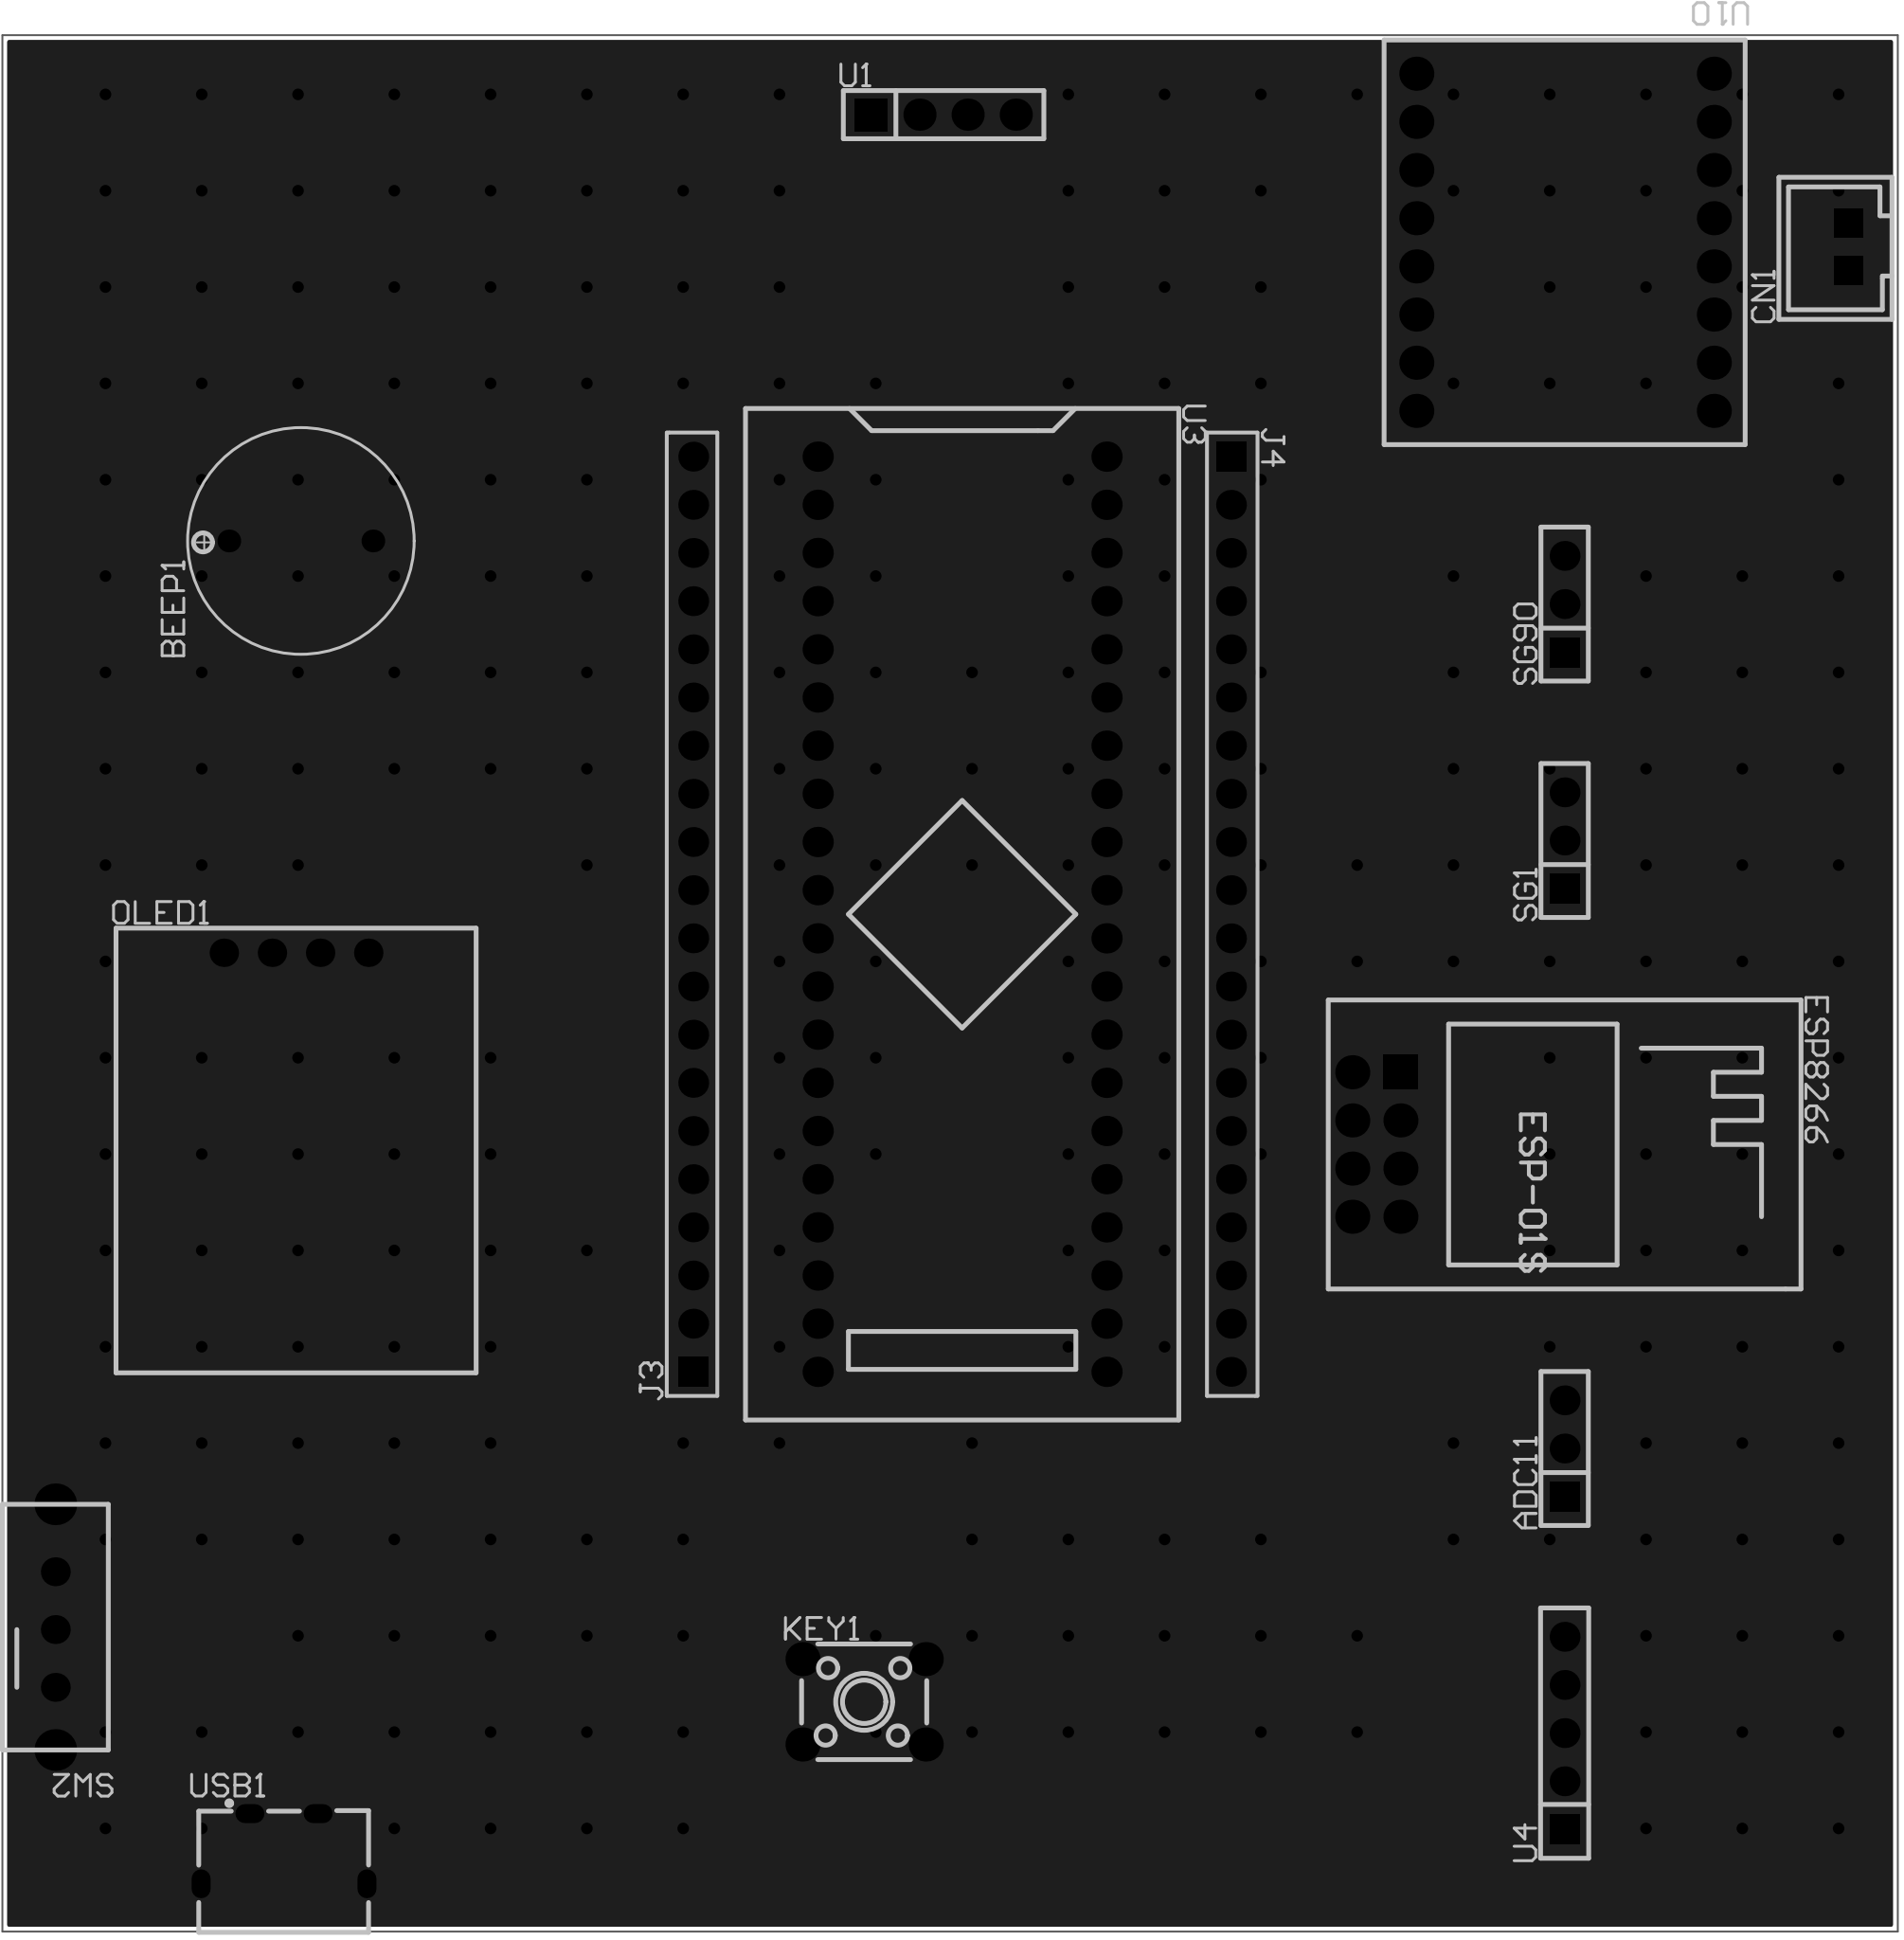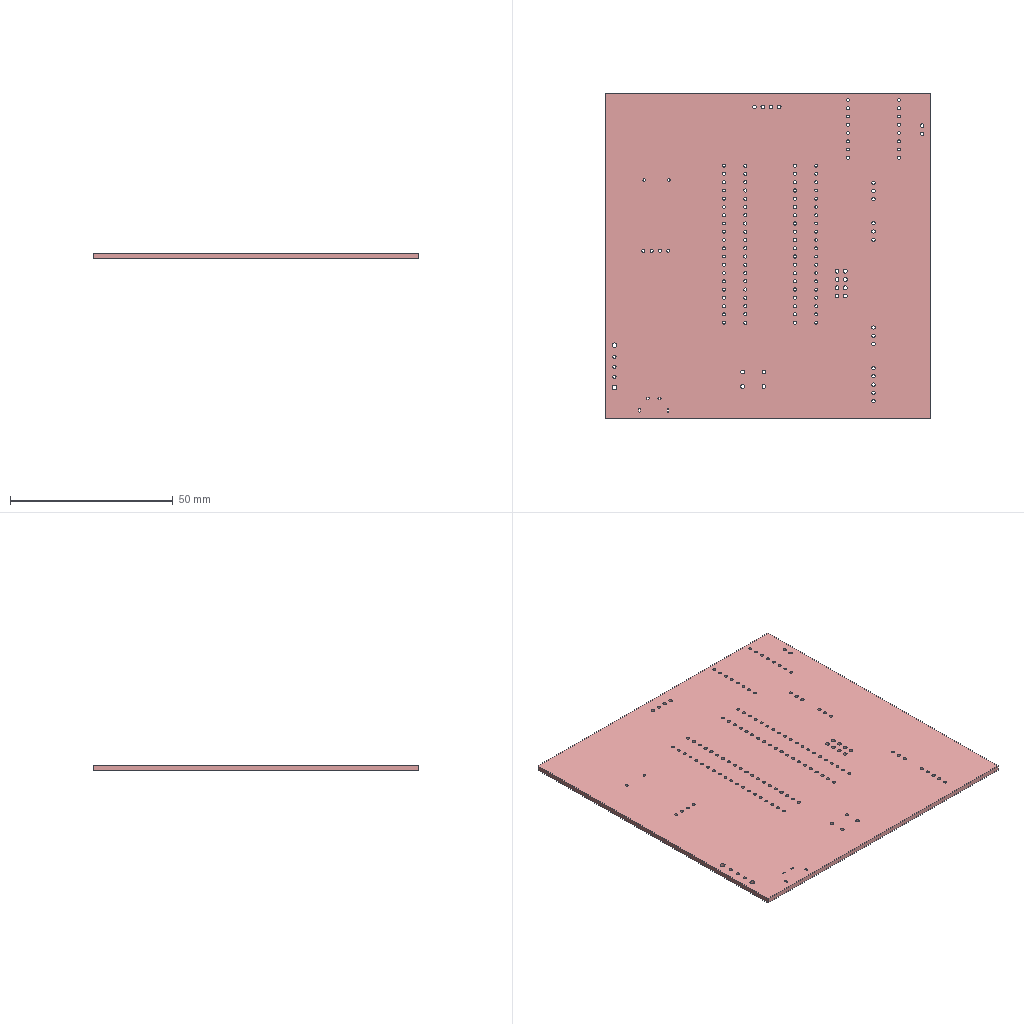Circuit board layout | Altium Designer | box 100 x 100 x 1.6 mm
Layer stack:
# Altium Designer layer stack of  (unit mm; dielectric type: 0 none, 1 core, 2 prepreg, 3 surface material)
index,name,kind,layer,copper_thickness_mm,dielectric_type,dielectric_thickness_mm,dielectric_material,dielectric_constant
0,Top Paste Mask Layer,other,,,,,,
1,Top Silkscreen Layer,other,,,,,,
2,Top Solder Mask Layer,dielectric,,,3,0.01,,3.3
3,Top Layer,copper,Top Layer,0.035,,,,
4,Dielectric1,dielectric,,,3,1.51,FR4,4.5
5,Bottom Layer,copper,Bottom Layer,0.035,,,,
6,Bottom Solder Mask Layer,dielectric,,,3,0.01,,3.3
7,Bottom Silkscreen Layer,other,,,,,,
8,Bottom Paste Mask Layer,other,,,,,,
# drill layer pairs: low layer,high layer
drill_pair,Top Layer,Bottom Layer
Part placement:
Designator,Comment,Layer,Footprint,Center-X(mm),Center-Y(mm),Rotation
ADC11,MQ135,TopLayer,HDR-TH_3P-P2.54-V-F,164.719,108.48,90
BEEP1,Buzzer,TopLayer,BUZ-TH_BD11.8-P7.60_XHXDZ-TMB12065,98.044,156.337,90
CN1,XH2.54-2PIN-straight pin,TopLayer,CONN-TH_XH2.54-2P,179.705,171.831,90
ESP8266,ESP-01S module,TopLayer,WIFIM-TH_ESP-01S,154.788,124.51,270
J3,HDR-M-2.54_1x20,TopLayer,HDR-M-2.54_1X20,118.745,136.652,90
J4,HDR-M-2.54_1x20,TopLayer,HDR-M-2.54_1X20,147.119,136.652,270
KEY1,K4-6×6_TH,TopLayer,KEY-TH_4P-L6.0-W6.0-P4.50-LS6.5,127.762,95.123,0
OLED1,0.96 OLED IIC COPY,TopLayer,OLED-TH_4P-L23.44-W19.0_ER-OLEDM0.66-1W-I2C,97.79,134.62,0
SG1,Servo,TopLayer,HDR-TH_3P-P2.54-V-F,164.719,140.541,90
SG90,Servo,TopLayer,HDR-TH_3P-P2.54-V-F,164.719,153.009,90
SW2,SK-12E12-G5,TopLayer,SW-TH_SK-12E12-G5,85.09,99.06,180
U1,HX711,TopLayer,HDR-TH_4P-P2.54-V-F,131.953,178.816,0
U3,STM32F103C8T6-Card,TopLayer,CONN-TH_L53.3-W22.9_STM32F103C8T6-CARD,132.932,136.652,270
U4,Clock DS1302,TopLayer,HDR-TH_5P-P2.54-V-F,164.719,93.472,90
U10,TB6612FNG,TopLayer,tb6612,164.744,172.085,180
USB1,KH-TYPE-C-2P,TopLayer,USB-SMD_KH-TYPE-C-2P,97.155,87.376,0
Pad and via stacks:
# Altium Designer via and pad stacks of  (unit mm). Each distinct definition once, with the count of objects using it.
# via: kind,start_layer,end_layer,hole_mm,diameter_mm,mode(0 simple;1 top-mid-bottom;2 full stack),diameter_per_layer,count,example_net
# pad: kind,layer,hole_mm,hole_type(0 round;1 square;2 slot),plating,top_size,top_shape(1 round;2 rect;3 octagon;9 rounded rect),mid_size,bottom_size,mode,footprint,size_per_layer,count,example
pad,Multi-Layer,1.02,0,plated,1.575x1.575,1,1.575x1.575,1.575x1.575,0,HDR-TH_3P-P2.54-V-F,,6,ADC11.3
pad,Multi-Layer,1.02,0,plated,1.575x1.575,2,1.575x1.575,1.575x1.575,0,HDR-TH_3P-P2.54-V-F,,3,ADC11.1
pad,Multi-Layer,0.801,0,plated,1.202x1.202,1,1.202x1.202,1.202x1.202,0,BUZ-TH_BD11.8-P7.60_XHXDZ-TMB12065,,2,BEEP1.1
pad,Multi-Layer,1,2,plated,1.524x1.524,2,1.524x1.524,1.524x1.524,0,CONN-TH_XH2.54-2P,,2,CN1.1
pad,Multi-Layer,1.2,0,plated,1.8x1.8,2,1.8x1.8,1.8x1.8,0,WIFIM-TH_ESP-01S,,1,ESP8266.1
pad,Multi-Layer,1.2,0,plated,1.8x1.8,1,1.8x1.8,1.8x1.8,0,WIFIM-TH_ESP-01S,,7,ESP8266.2
pad,Multi-Layer,0.889,0,plated,1.575x1.575,1,1.575x1.575,1.575x1.575,0,HDR-M-2.54_1X20,,38,J3.20
pad,Multi-Layer,0.889,0,plated,1.575x1.575,2,1.575x1.575,1.575x1.575,0,HDR-M-2.54_1X20,,2,J3.1
pad,Multi-Layer,1.1,0,plated,1.8x1.8,1,1.8x1.8,1.8x1.8,0,KEY-TH_4P-L6.0-W6.0-P4.50-LS6.5,,4,KEY1.4
pad,Multi-Layer,0.9,0,plated,1.5x1.5,1,1.5x1.5,1.5x1.5,0,OLED-TH_4P-L23.44-W19.0_ER-OLEDM0.66-1W-I2C,,4,OLED1.1
pad,Multi-Layer,1,0,plated,1.524x1.524,1,1.524x1.524,1.524x1.524,0,SW-TH_SK-12E12-G5,,3,SW2.2
pad,Multi-Layer,1.5,0,plated,2.2x2.2,1,2.2x2.2,2.2x2.2,0,SW-TH_SK-12E12-G5,,2,SW2.4
pad,Multi-Layer,1.1,0,plated,1.7x1.7,2,1.7x1.7,1.7x1.7,0,HDR-TH_4P-P2.54-V-F,,1,U1.1
pad,Multi-Layer,1.1,0,plated,1.7x1.7,1,1.7x1.7,1.7x1.7,0,HDR-TH_4P-P2.54-V-F,,3,U1.2
pad,Multi-Layer,1,0,plated,1.6x1.6,1,1.6x1.6,1.6x1.6,0,CONN-TH_L53.3-W22.9_STM32F103C8T6-CARD,,40,U3.1
pad,Multi-Layer,1.02,0,plated,1.575x1.575,1,1.575x1.575,1.575x1.575,0,HDR-TH_5P-P2.54-V-F,,4,U4.5
pad,Multi-Layer,1.02,0,plated,1.575x1.575,2,1.575x1.575,1.575x1.575,0,HDR-TH_5P-P2.54-V-F,,1,U4.1
pad,Multi-Layer,0.9,0,plated,1.8x1.8,1,1.8x1.8,1.8x1.8,0,tb6612,,16,U10.1
pad,Multi-Layer,0.45,2,plated,1x1.524,1,1x1.524,1x1.524,0,USB-SMD_KH-TYPE-C-2P,,2,USB1.1
pad,Multi-Layer,0.5,2,plated,1x1.524,1,1x1.524,1x1.524,0,USB-SMD_KH-TYPE-C-2P,,2,USB1.3
via,Top Layer,Bottom Layer,0.3048,0.61,0,,269,GND
Copper pours:
name,layer,net,type(0 solid;1 hatched;2 none)
Top Layer-GND,Top Layer,GND,0
Bottom Layer-GND,Bottom Layer,GND,0